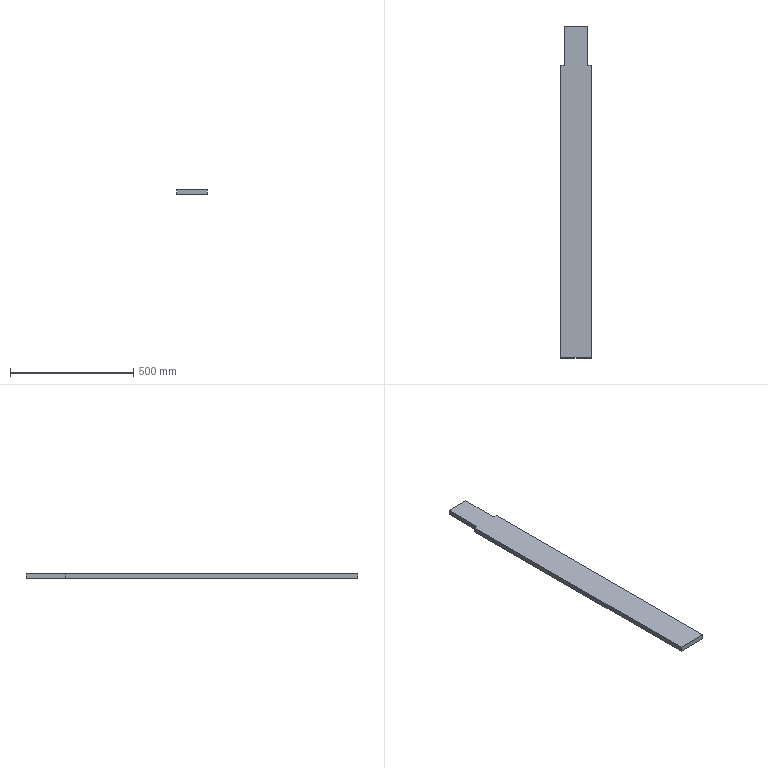Part | STEP file | 01 Counterweight block | 1 solid | 10 faces | box 124 x 1345 x 20 mm | volume 3242800 mm3 | plane 10
STEP:
#1=CARTESIAN_POINT('',(0.,0.,0.));
#2=DIRECTION('',(0.,0.,1.));
#3=DIRECTION('',(1.,0.,0.));
#4=AXIS2_PLACEMENT_3D('',#1,#2,#3);
#5=CARTESIAN_POINT('',(0.,1185.,0.));
#6=VERTEX_POINT('',#5);
#7=CARTESIAN_POINT('',(0.,0.,0.));
#8=VERTEX_POINT('',#7);
#9=CARTESIAN_POINT('',(0.,0.,0.));
#10=DIRECTION('',(0.,-1.,0.));
#11=VECTOR('',#10,1.);
#12=LINE('',#9,#11);
#13=CARTESIAN_POINT('',(0.,0.,20.));
#14=DIRECTION('',(1.,0.,0.));
#15=DIRECTION('',(0.,0.,-1.));
#16=AXIS2_PLACEMENT_3D('',#13,#14,#15);
#17=PLANE('',#16);
#18=CARTESIAN_POINT('',(20.,0.));
#19=DIRECTION('',(0.,-1.));
#20=VECTOR('',#19,1.);
#21=LINE('',#18,#20);
#22=(GEOMETRIC_REPRESENTATION_CONTEXT(2)PARAMETRIC_REPRESENTATION_CONTEXT()REPRESENTATION_CONTEXT('',''));
#23=DEFINITIONAL_REPRESENTATION('',(#21),#22);
#24=PCURVE('',#17,#23);
#25=CARTESIAN_POINT('',(0.,0.,0.));
#26=DIRECTION('',(0.,0.,1.));
#27=DIRECTION('',(1.,0.,0.));
#28=AXIS2_PLACEMENT_3D('',#25,#26,#27);
#29=PLANE('',#28);
#30=CARTESIAN_POINT('',(0.,0.));
#31=DIRECTION('',(0.,-1.));
#32=VECTOR('',#31,1.);
#33=LINE('',#30,#32);
#34=(GEOMETRIC_REPRESENTATION_CONTEXT(2)PARAMETRIC_REPRESENTATION_CONTEXT()REPRESENTATION_CONTEXT('',''));
#35=DEFINITIONAL_REPRESENTATION('',(#33),#34);
#36=PCURVE('',#29,#35);
#37=SURFACE_CURVE('',#12,(#24,#36),.PCURVE_S1.);
#38=EDGE_CURVE('',#6,#8,#37,.T.);
#39=ORIENTED_EDGE('',*,*,#38,.T.);
#40=CARTESIAN_POINT('',(0.,0.,20.));
#41=VERTEX_POINT('',#40);
#42=CARTESIAN_POINT('',(0.,0.,20.));
#43=DIRECTION('',(0.,0.,-1.));
#44=VECTOR('',#43,1.);
#45=LINE('',#42,#44);
#46=CARTESIAN_POINT('',(0.,0.));
#47=DIRECTION('',(1.,0.));
#48=VECTOR('',#47,1.);
#49=LINE('',#46,#48);
#50=(GEOMETRIC_REPRESENTATION_CONTEXT(2)PARAMETRIC_REPRESENTATION_CONTEXT()REPRESENTATION_CONTEXT('',''));
#51=DEFINITIONAL_REPRESENTATION('',(#49),#50);
#52=PCURVE('',#17,#51);
#53=CARTESIAN_POINT('',(0.,0.,20.));
#54=DIRECTION('',(0.,1.,0.));
#55=DIRECTION('',(0.,0.,1.));
#56=AXIS2_PLACEMENT_3D('',#53,#54,#55);
#57=PLANE('',#56);
#58=CARTESIAN_POINT('',(0.,0.));
#59=DIRECTION('',(-1.,0.));
#60=VECTOR('',#59,1.);
#61=LINE('',#58,#60);
#62=(GEOMETRIC_REPRESENTATION_CONTEXT(2)PARAMETRIC_REPRESENTATION_CONTEXT()REPRESENTATION_CONTEXT('',''));
#63=DEFINITIONAL_REPRESENTATION('',(#61),#62);
#64=PCURVE('',#57,#63);
#65=SURFACE_CURVE('',#45,(#52,#64),.PCURVE_S1.);
#66=EDGE_CURVE('',#41,#8,#65,.T.);
#67=ORIENTED_EDGE('',*,*,#66,.F.);
#68=CARTESIAN_POINT('',(0.,1185.,20.));
#69=VERTEX_POINT('',#68);
#70=CARTESIAN_POINT('',(0.,0.,20.));
#71=DIRECTION('',(0.,-1.,0.));
#72=VECTOR('',#71,1.);
#73=LINE('',#70,#72);
#74=CARTESIAN_POINT('',(0.,0.));
#75=DIRECTION('',(0.,-1.));
#76=VECTOR('',#75,1.);
#77=LINE('',#74,#76);
#78=(GEOMETRIC_REPRESENTATION_CONTEXT(2)PARAMETRIC_REPRESENTATION_CONTEXT()REPRESENTATION_CONTEXT('',''));
#79=DEFINITIONAL_REPRESENTATION('',(#77),#78);
#80=PCURVE('',#17,#79);
#81=CARTESIAN_POINT('',(0.,0.,20.));
#82=DIRECTION('',(0.,0.,1.));
#83=DIRECTION('',(1.,0.,0.));
#84=AXIS2_PLACEMENT_3D('',#81,#82,#83);
#85=PLANE('',#84);
#86=CARTESIAN_POINT('',(0.,0.));
#87=DIRECTION('',(0.,-1.));
#88=VECTOR('',#87,1.);
#89=LINE('',#86,#88);
#90=(GEOMETRIC_REPRESENTATION_CONTEXT(2)PARAMETRIC_REPRESENTATION_CONTEXT()REPRESENTATION_CONTEXT('',''));
#91=DEFINITIONAL_REPRESENTATION('',(#89),#90);
#92=PCURVE('',#85,#91);
#93=SURFACE_CURVE('',#73,(#80,#92),.PCURVE_S1.);
#94=EDGE_CURVE('',#69,#41,#93,.T.);
#95=ORIENTED_EDGE('',*,*,#94,.F.);
#96=CARTESIAN_POINT('',(0.,1185.,20.));
#97=DIRECTION('',(0.,0.,-1.));
#98=VECTOR('',#97,1.);
#99=LINE('',#96,#98);
#100=CARTESIAN_POINT('',(0.,1185.));
#101=DIRECTION('',(1.,0.));
#102=VECTOR('',#101,1.);
#103=LINE('',#100,#102);
#104=(GEOMETRIC_REPRESENTATION_CONTEXT(2)PARAMETRIC_REPRESENTATION_CONTEXT()REPRESENTATION_CONTEXT('',''));
#105=DEFINITIONAL_REPRESENTATION('',(#103),#104);
#106=PCURVE('',#17,#105);
#107=CARTESIAN_POINT('',(14.5,1185.,20.));
#108=DIRECTION('',(0.,-1.,0.));
#109=DIRECTION('',(0.,0.,-1.));
#110=AXIS2_PLACEMENT_3D('',#107,#108,#109);
#111=PLANE('',#110);
#112=CARTESIAN_POINT('',(0.,-14.5));
#113=DIRECTION('',(1.,0.));
#114=VECTOR('',#113,1.);
#115=LINE('',#112,#114);
#116=(GEOMETRIC_REPRESENTATION_CONTEXT(2)PARAMETRIC_REPRESENTATION_CONTEXT()REPRESENTATION_CONTEXT('',''));
#117=DEFINITIONAL_REPRESENTATION('',(#115),#116);
#118=PCURVE('',#111,#117);
#119=SURFACE_CURVE('',#99,(#106,#118),.PCURVE_S1.);
#120=EDGE_CURVE('',#69,#6,#119,.T.);
#121=ORIENTED_EDGE('',*,*,#120,.T.);
#122=EDGE_LOOP('',(#39,#67,#95,#121));
#123=FACE_BOUND('',#122,.T.);
#124=ADVANCED_FACE('',(#123),#17,.F.);
#125=CARTESIAN_POINT('',(124.,0.,0.));
#126=VERTEX_POINT('',#125);
#127=CARTESIAN_POINT('',(0.,0.,0.));
#128=DIRECTION('',(1.,0.,0.));
#129=VECTOR('',#128,1.);
#130=LINE('',#127,#129);
#131=CARTESIAN_POINT('',(-20.,0.));
#132=DIRECTION('',(0.,1.));
#133=VECTOR('',#132,1.);
#134=LINE('',#131,#133);
#135=(GEOMETRIC_REPRESENTATION_CONTEXT(2)PARAMETRIC_REPRESENTATION_CONTEXT()REPRESENTATION_CONTEXT('',''));
#136=DEFINITIONAL_REPRESENTATION('',(#134),#135);
#137=PCURVE('',#57,#136);
#138=CARTESIAN_POINT('',(0.,0.));
#139=DIRECTION('',(1.,0.));
#140=VECTOR('',#139,1.);
#141=LINE('',#138,#140);
#142=(GEOMETRIC_REPRESENTATION_CONTEXT(2)PARAMETRIC_REPRESENTATION_CONTEXT()REPRESENTATION_CONTEXT('',''));
#143=DEFINITIONAL_REPRESENTATION('',(#141),#142);
#144=PCURVE('',#29,#143);
#145=SURFACE_CURVE('',#130,(#137,#144),.PCURVE_S1.);
#146=EDGE_CURVE('',#8,#126,#145,.T.);
#147=ORIENTED_EDGE('',*,*,#146,.T.);
#148=CARTESIAN_POINT('',(124.,0.,20.));
#149=VERTEX_POINT('',#148);
#150=CARTESIAN_POINT('',(124.,0.,20.));
#151=DIRECTION('',(0.,0.,-1.));
#152=VECTOR('',#151,1.);
#153=LINE('',#150,#152);
#154=CARTESIAN_POINT('',(0.,124.));
#155=DIRECTION('',(-1.,0.));
#156=VECTOR('',#155,1.);
#157=LINE('',#154,#156);
#158=(GEOMETRIC_REPRESENTATION_CONTEXT(2)PARAMETRIC_REPRESENTATION_CONTEXT()REPRESENTATION_CONTEXT('',''));
#159=DEFINITIONAL_REPRESENTATION('',(#157),#158);
#160=PCURVE('',#57,#159);
#161=CARTESIAN_POINT('',(124.,0.,20.));
#162=DIRECTION('',(-1.,0.,0.));
#163=DIRECTION('',(0.,0.,1.));
#164=AXIS2_PLACEMENT_3D('',#161,#162,#163);
#165=PLANE('',#164);
#166=CARTESIAN_POINT('',(0.,0.));
#167=DIRECTION('',(-1.,0.));
#168=VECTOR('',#167,1.);
#169=LINE('',#166,#168);
#170=(GEOMETRIC_REPRESENTATION_CONTEXT(2)PARAMETRIC_REPRESENTATION_CONTEXT()REPRESENTATION_CONTEXT('',''));
#171=DEFINITIONAL_REPRESENTATION('',(#169),#170);
#172=PCURVE('',#165,#171);
#173=SURFACE_CURVE('',#153,(#160,#172),.PCURVE_S1.);
#174=EDGE_CURVE('',#149,#126,#173,.T.);
#175=ORIENTED_EDGE('',*,*,#174,.F.);
#176=CARTESIAN_POINT('',(0.,0.,20.));
#177=DIRECTION('',(1.,0.,0.));
#178=VECTOR('',#177,1.);
#179=LINE('',#176,#178);
#180=CARTESIAN_POINT('',(0.,0.));
#181=DIRECTION('',(0.,1.));
#182=VECTOR('',#181,1.);
#183=LINE('',#180,#182);
#184=(GEOMETRIC_REPRESENTATION_CONTEXT(2)PARAMETRIC_REPRESENTATION_CONTEXT()REPRESENTATION_CONTEXT('',''));
#185=DEFINITIONAL_REPRESENTATION('',(#183),#184);
#186=PCURVE('',#57,#185);
#187=CARTESIAN_POINT('',(0.,0.));
#188=DIRECTION('',(1.,0.));
#189=VECTOR('',#188,1.);
#190=LINE('',#187,#189);
#191=(GEOMETRIC_REPRESENTATION_CONTEXT(2)PARAMETRIC_REPRESENTATION_CONTEXT()REPRESENTATION_CONTEXT('',''));
#192=DEFINITIONAL_REPRESENTATION('',(#190),#191);
#193=PCURVE('',#85,#192);
#194=SURFACE_CURVE('',#179,(#186,#193),.PCURVE_S1.);
#195=EDGE_CURVE('',#41,#149,#194,.T.);
#196=ORIENTED_EDGE('',*,*,#195,.F.);
#197=ORIENTED_EDGE('',*,*,#66,.T.);
#198=EDGE_LOOP('',(#147,#175,#196,#197));
#199=FACE_BOUND('',#198,.T.);
#200=ADVANCED_FACE('',(#199),#57,.F.);
#201=CARTESIAN_POINT('',(124.,1185.,0.));
#202=VERTEX_POINT('',#201);
#203=CARTESIAN_POINT('',(124.,0.,0.));
#204=DIRECTION('',(0.,1.,0.));
#205=VECTOR('',#204,1.);
#206=LINE('',#203,#205);
#207=CARTESIAN_POINT('',(-20.,0.));
#208=DIRECTION('',(0.,1.));
#209=VECTOR('',#208,1.);
#210=LINE('',#207,#209);
#211=(GEOMETRIC_REPRESENTATION_CONTEXT(2)PARAMETRIC_REPRESENTATION_CONTEXT()REPRESENTATION_CONTEXT('',''));
#212=DEFINITIONAL_REPRESENTATION('',(#210),#211);
#213=PCURVE('',#165,#212);
#214=CARTESIAN_POINT('',(124.,0.));
#215=DIRECTION('',(0.,1.));
#216=VECTOR('',#215,1.);
#217=LINE('',#214,#216);
#218=(GEOMETRIC_REPRESENTATION_CONTEXT(2)PARAMETRIC_REPRESENTATION_CONTEXT()REPRESENTATION_CONTEXT('',''));
#219=DEFINITIONAL_REPRESENTATION('',(#217),#218);
#220=PCURVE('',#29,#219);
#221=SURFACE_CURVE('',#206,(#213,#220),.PCURVE_S1.);
#222=EDGE_CURVE('',#126,#202,#221,.T.);
#223=ORIENTED_EDGE('',*,*,#222,.T.);
#224=CARTESIAN_POINT('',(124.,1185.,20.));
#225=VERTEX_POINT('',#224);
#226=CARTESIAN_POINT('',(124.,1185.,20.));
#227=DIRECTION('',(0.,0.,-1.));
#228=VECTOR('',#227,1.);
#229=LINE('',#226,#228);
#230=CARTESIAN_POINT('',(0.,1185.));
#231=DIRECTION('',(-1.,0.));
#232=VECTOR('',#231,1.);
#233=LINE('',#230,#232);
#234=(GEOMETRIC_REPRESENTATION_CONTEXT(2)PARAMETRIC_REPRESENTATION_CONTEXT()REPRESENTATION_CONTEXT('',''));
#235=DEFINITIONAL_REPRESENTATION('',(#233),#234);
#236=PCURVE('',#165,#235);
#237=CARTESIAN_POINT('',(109.5,1185.,20.));
#238=DIRECTION('',(0.,-1.,0.));
#239=DIRECTION('',(0.,0.,-1.));
#240=AXIS2_PLACEMENT_3D('',#237,#238,#239);
#241=PLANE('',#240);
#242=CARTESIAN_POINT('',(0.,14.5));
#243=DIRECTION('',(1.,0.));
#244=VECTOR('',#243,1.);
#245=LINE('',#242,#244);
#246=(GEOMETRIC_REPRESENTATION_CONTEXT(2)PARAMETRIC_REPRESENTATION_CONTEXT()REPRESENTATION_CONTEXT('',''));
#247=DEFINITIONAL_REPRESENTATION('',(#245),#246);
#248=PCURVE('',#241,#247);
#249=SURFACE_CURVE('',#229,(#236,#248),.PCURVE_S1.);
#250=EDGE_CURVE('',#225,#202,#249,.T.);
#251=ORIENTED_EDGE('',*,*,#250,.F.);
#252=CARTESIAN_POINT('',(124.,0.,20.));
#253=DIRECTION('',(0.,1.,0.));
#254=VECTOR('',#253,1.);
#255=LINE('',#252,#254);
#256=CARTESIAN_POINT('',(0.,0.));
#257=DIRECTION('',(0.,1.));
#258=VECTOR('',#257,1.);
#259=LINE('',#256,#258);
#260=(GEOMETRIC_REPRESENTATION_CONTEXT(2)PARAMETRIC_REPRESENTATION_CONTEXT()REPRESENTATION_CONTEXT('',''));
#261=DEFINITIONAL_REPRESENTATION('',(#259),#260);
#262=PCURVE('',#165,#261);
#263=CARTESIAN_POINT('',(124.,0.));
#264=DIRECTION('',(0.,1.));
#265=VECTOR('',#264,1.);
#266=LINE('',#263,#265);
#267=(GEOMETRIC_REPRESENTATION_CONTEXT(2)PARAMETRIC_REPRESENTATION_CONTEXT()REPRESENTATION_CONTEXT('',''));
#268=DEFINITIONAL_REPRESENTATION('',(#266),#267);
#269=PCURVE('',#85,#268);
#270=SURFACE_CURVE('',#255,(#262,#269),.PCURVE_S1.);
#271=EDGE_CURVE('',#149,#225,#270,.T.);
#272=ORIENTED_EDGE('',*,*,#271,.F.);
#273=ORIENTED_EDGE('',*,*,#174,.T.);
#274=EDGE_LOOP('',(#223,#251,#272,#273));
#275=FACE_BOUND('',#274,.T.);
#276=ADVANCED_FACE('',(#275),#165,.F.);
#277=CARTESIAN_POINT('',(109.5,1185.,0.));
#278=VERTEX_POINT('',#277);
#279=CARTESIAN_POINT('',(109.5,1185.,0.));
#280=DIRECTION('',(-1.,0.,0.));
#281=VECTOR('',#280,1.);
#282=LINE('',#279,#281);
#283=CARTESIAN_POINT('',(20.,0.));
#284=DIRECTION('',(0.,-1.));
#285=VECTOR('',#284,1.);
#286=LINE('',#283,#285);
#287=(GEOMETRIC_REPRESENTATION_CONTEXT(2)PARAMETRIC_REPRESENTATION_CONTEXT()REPRESENTATION_CONTEXT('',''));
#288=DEFINITIONAL_REPRESENTATION('',(#286),#287);
#289=PCURVE('',#241,#288);
#290=CARTESIAN_POINT('',(109.5,1185.));
#291=DIRECTION('',(-1.,0.));
#292=VECTOR('',#291,1.);
#293=LINE('',#290,#292);
#294=(GEOMETRIC_REPRESENTATION_CONTEXT(2)PARAMETRIC_REPRESENTATION_CONTEXT()REPRESENTATION_CONTEXT('',''));
#295=DEFINITIONAL_REPRESENTATION('',(#293),#294);
#296=PCURVE('',#29,#295);
#297=SURFACE_CURVE('',#282,(#289,#296),.PCURVE_S1.);
#298=EDGE_CURVE('',#202,#278,#297,.T.);
#299=ORIENTED_EDGE('',*,*,#298,.T.);
#300=CARTESIAN_POINT('',(109.5,1185.,20.));
#301=VERTEX_POINT('',#300);
#302=CARTESIAN_POINT('',(109.5,1185.,20.));
#303=DIRECTION('',(0.,0.,-1.));
#304=VECTOR('',#303,1.);
#305=LINE('',#302,#304);
#306=CARTESIAN_POINT('',(0.,0.));
#307=DIRECTION('',(1.,0.));
#308=VECTOR('',#307,1.);
#309=LINE('',#306,#308);
#310=(GEOMETRIC_REPRESENTATION_CONTEXT(2)PARAMETRIC_REPRESENTATION_CONTEXT()REPRESENTATION_CONTEXT('',''));
#311=DEFINITIONAL_REPRESENTATION('',(#309),#310);
#312=PCURVE('',#241,#311);
#313=CARTESIAN_POINT('',(109.5,1345.,20.));
#314=DIRECTION('',(-1.,0.,0.));
#315=DIRECTION('',(0.,0.,1.));
#316=AXIS2_PLACEMENT_3D('',#313,#314,#315);
#317=PLANE('',#316);
#318=CARTESIAN_POINT('',(0.,-160.));
#319=DIRECTION('',(-1.,0.));
#320=VECTOR('',#319,1.);
#321=LINE('',#318,#320);
#322=(GEOMETRIC_REPRESENTATION_CONTEXT(2)PARAMETRIC_REPRESENTATION_CONTEXT()REPRESENTATION_CONTEXT('',''));
#323=DEFINITIONAL_REPRESENTATION('',(#321),#322);
#324=PCURVE('',#317,#323);
#325=SURFACE_CURVE('',#305,(#312,#324),.PCURVE_S1.);
#326=EDGE_CURVE('',#301,#278,#325,.T.);
#327=ORIENTED_EDGE('',*,*,#326,.F.);
#328=CARTESIAN_POINT('',(109.5,1185.,20.));
#329=DIRECTION('',(-1.,0.,0.));
#330=VECTOR('',#329,1.);
#331=LINE('',#328,#330);
#332=CARTESIAN_POINT('',(0.,0.));
#333=DIRECTION('',(0.,-1.));
#334=VECTOR('',#333,1.);
#335=LINE('',#332,#334);
#336=(GEOMETRIC_REPRESENTATION_CONTEXT(2)PARAMETRIC_REPRESENTATION_CONTEXT()REPRESENTATION_CONTEXT('',''));
#337=DEFINITIONAL_REPRESENTATION('',(#335),#336);
#338=PCURVE('',#241,#337);
#339=CARTESIAN_POINT('',(109.5,1185.));
#340=DIRECTION('',(-1.,0.));
#341=VECTOR('',#340,1.);
#342=LINE('',#339,#341);
#343=(GEOMETRIC_REPRESENTATION_CONTEXT(2)PARAMETRIC_REPRESENTATION_CONTEXT()REPRESENTATION_CONTEXT('',''));
#344=DEFINITIONAL_REPRESENTATION('',(#342),#343);
#345=PCURVE('',#85,#344);
#346=SURFACE_CURVE('',#331,(#338,#345),.PCURVE_S1.);
#347=EDGE_CURVE('',#225,#301,#346,.T.);
#348=ORIENTED_EDGE('',*,*,#347,.F.);
#349=ORIENTED_EDGE('',*,*,#250,.T.);
#350=EDGE_LOOP('',(#299,#327,#348,#349));
#351=FACE_BOUND('',#350,.T.);
#352=ADVANCED_FACE('',(#351),#241,.F.);
#353=CARTESIAN_POINT('',(109.5,1345.,0.));
#354=VERTEX_POINT('',#353);
#355=CARTESIAN_POINT('',(109.5,1345.,0.));
#356=DIRECTION('',(0.,1.,0.));
#357=VECTOR('',#356,1.);
#358=LINE('',#355,#357);
#359=CARTESIAN_POINT('',(-20.,0.));
#360=DIRECTION('',(0.,1.));
#361=VECTOR('',#360,1.);
#362=LINE('',#359,#361);
#363=(GEOMETRIC_REPRESENTATION_CONTEXT(2)PARAMETRIC_REPRESENTATION_CONTEXT()REPRESENTATION_CONTEXT('',''));
#364=DEFINITIONAL_REPRESENTATION('',(#362),#363);
#365=PCURVE('',#317,#364);
#366=CARTESIAN_POINT('',(109.5,1345.));
#367=DIRECTION('',(0.,1.));
#368=VECTOR('',#367,1.);
#369=LINE('',#366,#368);
#370=(GEOMETRIC_REPRESENTATION_CONTEXT(2)PARAMETRIC_REPRESENTATION_CONTEXT()REPRESENTATION_CONTEXT('',''));
#371=DEFINITIONAL_REPRESENTATION('',(#369),#370);
#372=PCURVE('',#29,#371);
#373=SURFACE_CURVE('',#358,(#365,#372),.PCURVE_S1.);
#374=EDGE_CURVE('',#278,#354,#373,.T.);
#375=ORIENTED_EDGE('',*,*,#374,.T.);
#376=CARTESIAN_POINT('',(109.5,1345.,20.));
#377=VERTEX_POINT('',#376);
#378=CARTESIAN_POINT('',(109.5,1345.,20.));
#379=DIRECTION('',(0.,0.,-1.));
#380=VECTOR('',#379,1.);
#381=LINE('',#378,#380);
#382=CARTESIAN_POINT('',(0.,0.));
#383=DIRECTION('',(-1.,0.));
#384=VECTOR('',#383,1.);
#385=LINE('',#382,#384);
#386=(GEOMETRIC_REPRESENTATION_CONTEXT(2)PARAMETRIC_REPRESENTATION_CONTEXT()REPRESENTATION_CONTEXT('',''));
#387=DEFINITIONAL_REPRESENTATION('',(#385),#386);
#388=PCURVE('',#317,#387);
#389=CARTESIAN_POINT('',(14.5,1345.,20.));
#390=DIRECTION('',(0.,-1.,0.));
#391=DIRECTION('',(0.,0.,-1.));
#392=AXIS2_PLACEMENT_3D('',#389,#390,#391);
#393=PLANE('',#392);
#394=CARTESIAN_POINT('',(0.,95.));
#395=DIRECTION('',(1.,0.));
#396=VECTOR('',#395,1.);
#397=LINE('',#394,#396);
#398=(GEOMETRIC_REPRESENTATION_CONTEXT(2)PARAMETRIC_REPRESENTATION_CONTEXT()REPRESENTATION_CONTEXT('',''));
#399=DEFINITIONAL_REPRESENTATION('',(#397),#398);
#400=PCURVE('',#393,#399);
#401=SURFACE_CURVE('',#381,(#388,#400),.PCURVE_S1.);
#402=EDGE_CURVE('',#377,#354,#401,.T.);
#403=ORIENTED_EDGE('',*,*,#402,.F.);
#404=CARTESIAN_POINT('',(109.5,1345.,20.));
#405=DIRECTION('',(0.,1.,0.));
#406=VECTOR('',#405,1.);
#407=LINE('',#404,#406);
#408=CARTESIAN_POINT('',(0.,0.));
#409=DIRECTION('',(0.,1.));
#410=VECTOR('',#409,1.);
#411=LINE('',#408,#410);
#412=(GEOMETRIC_REPRESENTATION_CONTEXT(2)PARAMETRIC_REPRESENTATION_CONTEXT()REPRESENTATION_CONTEXT('',''));
#413=DEFINITIONAL_REPRESENTATION('',(#411),#412);
#414=PCURVE('',#317,#413);
#415=CARTESIAN_POINT('',(109.5,1345.));
#416=DIRECTION('',(0.,1.));
#417=VECTOR('',#416,1.);
#418=LINE('',#415,#417);
#419=(GEOMETRIC_REPRESENTATION_CONTEXT(2)PARAMETRIC_REPRESENTATION_CONTEXT()REPRESENTATION_CONTEXT('',''));
#420=DEFINITIONAL_REPRESENTATION('',(#418),#419);
#421=PCURVE('',#85,#420);
#422=SURFACE_CURVE('',#407,(#414,#421),.PCURVE_S1.);
#423=EDGE_CURVE('',#301,#377,#422,.T.);
#424=ORIENTED_EDGE('',*,*,#423,.F.);
#425=ORIENTED_EDGE('',*,*,#326,.T.);
#426=EDGE_LOOP('',(#375,#403,#424,#425));
#427=FACE_BOUND('',#426,.T.);
#428=ADVANCED_FACE('',(#427),#317,.F.);
#429=CARTESIAN_POINT('',(14.5,1345.,0.));
#430=VERTEX_POINT('',#429);
#431=CARTESIAN_POINT('',(14.5,1345.,0.));
#432=DIRECTION('',(-1.,0.,0.));
#433=VECTOR('',#432,1.);
#434=LINE('',#431,#433);
#435=CARTESIAN_POINT('',(20.,0.));
#436=DIRECTION('',(0.,-1.));
#437=VECTOR('',#436,1.);
#438=LINE('',#435,#437);
#439=(GEOMETRIC_REPRESENTATION_CONTEXT(2)PARAMETRIC_REPRESENTATION_CONTEXT()REPRESENTATION_CONTEXT('',''));
#440=DEFINITIONAL_REPRESENTATION('',(#438),#439);
#441=PCURVE('',#393,#440);
#442=CARTESIAN_POINT('',(14.5,1345.));
#443=DIRECTION('',(-1.,0.));
#444=VECTOR('',#443,1.);
#445=LINE('',#442,#444);
#446=(GEOMETRIC_REPRESENTATION_CONTEXT(2)PARAMETRIC_REPRESENTATION_CONTEXT()REPRESENTATION_CONTEXT('',''));
#447=DEFINITIONAL_REPRESENTATION('',(#445),#446);
#448=PCURVE('',#29,#447);
#449=SURFACE_CURVE('',#434,(#441,#448),.PCURVE_S1.);
#450=EDGE_CURVE('',#354,#430,#449,.T.);
#451=ORIENTED_EDGE('',*,*,#450,.T.);
#452=CARTESIAN_POINT('',(14.5,1345.,20.));
#453=VERTEX_POINT('',#452);
#454=CARTESIAN_POINT('',(14.5,1345.,20.));
#455=DIRECTION('',(0.,0.,-1.));
#456=VECTOR('',#455,1.);
#457=LINE('',#454,#456);
#458=CARTESIAN_POINT('',(0.,0.));
#459=DIRECTION('',(1.,0.));
#460=VECTOR('',#459,1.);
#461=LINE('',#458,#460);
#462=(GEOMETRIC_REPRESENTATION_CONTEXT(2)PARAMETRIC_REPRESENTATION_CONTEXT()REPRESENTATION_CONTEXT('',''));
#463=DEFINITIONAL_REPRESENTATION('',(#461),#462);
#464=PCURVE('',#393,#463);
#465=CARTESIAN_POINT('',(14.5,1345.,20.));
#466=DIRECTION('',(1.,0.,0.));
#467=DIRECTION('',(0.,1.,0.));
#468=AXIS2_PLACEMENT_3D('',#465,#466,#467);
#469=PLANE('',#468);
#470=CARTESIAN_POINT('',(0.,0.));
#471=DIRECTION('',(0.,-1.));
#472=VECTOR('',#471,1.);
#473=LINE('',#470,#472);
#474=(GEOMETRIC_REPRESENTATION_CONTEXT(2)PARAMETRIC_REPRESENTATION_CONTEXT()REPRESENTATION_CONTEXT('',''));
#475=DEFINITIONAL_REPRESENTATION('',(#473),#474);
#476=PCURVE('',#469,#475);
#477=SURFACE_CURVE('',#457,(#464,#476),.PCURVE_S1.);
#478=EDGE_CURVE('',#453,#430,#477,.T.);
#479=ORIENTED_EDGE('',*,*,#478,.F.);
#480=CARTESIAN_POINT('',(14.5,1345.,20.));
#481=DIRECTION('',(-1.,0.,0.));
#482=VECTOR('',#481,1.);
#483=LINE('',#480,#482);
#484=CARTESIAN_POINT('',(0.,0.));
#485=DIRECTION('',(0.,-1.));
#486=VECTOR('',#485,1.);
#487=LINE('',#484,#486);
#488=(GEOMETRIC_REPRESENTATION_CONTEXT(2)PARAMETRIC_REPRESENTATION_CONTEXT()REPRESENTATION_CONTEXT('',''));
#489=DEFINITIONAL_REPRESENTATION('',(#487),#488);
#490=PCURVE('',#393,#489);
#491=CARTESIAN_POINT('',(14.5,1345.));
#492=DIRECTION('',(-1.,0.));
#493=VECTOR('',#492,1.);
#494=LINE('',#491,#493);
#495=(GEOMETRIC_REPRESENTATION_CONTEXT(2)PARAMETRIC_REPRESENTATION_CONTEXT()REPRESENTATION_CONTEXT('',''));
#496=DEFINITIONAL_REPRESENTATION('',(#494),#495);
#497=PCURVE('',#85,#496);
#498=SURFACE_CURVE('',#483,(#490,#497),.PCURVE_S1.);
#499=EDGE_CURVE('',#377,#453,#498,.T.);
#500=ORIENTED_EDGE('',*,*,#499,.F.);
#501=ORIENTED_EDGE('',*,*,#402,.T.);
#502=EDGE_LOOP('',(#451,#479,#500,#501));
#503=FACE_BOUND('',#502,.T.);
#504=ADVANCED_FACE('',(#503),#393,.F.);
#505=CARTESIAN_POINT('',(14.5,1185.,0.));
#506=VERTEX_POINT('',#505);
#507=CARTESIAN_POINT('',(14.5,1345.,0.));
#508=DIRECTION('',(0.,-1.,0.));
#509=VECTOR('',#508,1.);
#510=LINE('',#507,#509);
#511=CARTESIAN_POINT('',(0.,-20.));
#512=DIRECTION('',(-1.,0.));
#513=VECTOR('',#512,1.);
#514=LINE('',#511,#513);
#515=(GEOMETRIC_REPRESENTATION_CONTEXT(2)PARAMETRIC_REPRESENTATION_CONTEXT()REPRESENTATION_CONTEXT('',''));
#516=DEFINITIONAL_REPRESENTATION('',(#514),#515);
#517=PCURVE('',#469,#516);
#518=CARTESIAN_POINT('',(14.5,1345.));
#519=DIRECTION('',(0.,-1.));
#520=VECTOR('',#519,1.);
#521=LINE('',#518,#520);
#522=(GEOMETRIC_REPRESENTATION_CONTEXT(2)PARAMETRIC_REPRESENTATION_CONTEXT()REPRESENTATION_CONTEXT('',''));
#523=DEFINITIONAL_REPRESENTATION('',(#521),#522);
#524=PCURVE('',#29,#523);
#525=SURFACE_CURVE('',#510,(#517,#524),.PCURVE_S1.);
#526=EDGE_CURVE('',#430,#506,#525,.T.);
#527=ORIENTED_EDGE('',*,*,#526,.T.);
#528=CARTESIAN_POINT('',(14.5,1185.,20.));
#529=VERTEX_POINT('',#528);
#530=CARTESIAN_POINT('',(14.5,1185.,20.));
#531=DIRECTION('',(0.,0.,-1.));
#532=VECTOR('',#531,1.);
#533=LINE('',#530,#532);
#534=CARTESIAN_POINT('',(-160.,0.));
#535=DIRECTION('',(0.,-1.));
#536=VECTOR('',#535,1.);
#537=LINE('',#534,#536);
#538=(GEOMETRIC_REPRESENTATION_CONTEXT(2)PARAMETRIC_REPRESENTATION_CONTEXT()REPRESENTATION_CONTEXT('',''));
#539=DEFINITIONAL_REPRESENTATION('',(#537),#538);
#540=PCURVE('',#469,#539);
#541=CARTESIAN_POINT('',(0.,0.));
#542=DIRECTION('',(1.,0.));
#543=VECTOR('',#542,1.);
#544=LINE('',#541,#543);
#545=(GEOMETRIC_REPRESENTATION_CONTEXT(2)PARAMETRIC_REPRESENTATION_CONTEXT()REPRESENTATION_CONTEXT('',''));
#546=DEFINITIONAL_REPRESENTATION('',(#544),#545);
#547=PCURVE('',#111,#546);
#548=SURFACE_CURVE('',#533,(#540,#547),.PCURVE_S1.);
#549=EDGE_CURVE('',#529,#506,#548,.T.);
#550=ORIENTED_EDGE('',*,*,#549,.F.);
#551=CARTESIAN_POINT('',(14.5,1345.,20.));
#552=DIRECTION('',(0.,-1.,0.));
#553=VECTOR('',#552,1.);
#554=LINE('',#551,#553);
#555=CARTESIAN_POINT('',(0.,0.));
#556=DIRECTION('',(-1.,0.));
#557=VECTOR('',#556,1.);
#558=LINE('',#555,#557);
#559=(GEOMETRIC_REPRESENTATION_CONTEXT(2)PARAMETRIC_REPRESENTATION_CONTEXT()REPRESENTATION_CONTEXT('',''));
#560=DEFINITIONAL_REPRESENTATION('',(#558),#559);
#561=PCURVE('',#469,#560);
#562=CARTESIAN_POINT('',(14.5,1345.));
#563=DIRECTION('',(0.,-1.));
#564=VECTOR('',#563,1.);
#565=LINE('',#562,#564);
#566=(GEOMETRIC_REPRESENTATION_CONTEXT(2)PARAMETRIC_REPRESENTATION_CONTEXT()REPRESENTATION_CONTEXT('',''));
#567=DEFINITIONAL_REPRESENTATION('',(#565),#566);
#568=PCURVE('',#85,#567);
#569=SURFACE_CURVE('',#554,(#561,#568),.PCURVE_S1.);
#570=EDGE_CURVE('',#453,#529,#569,.T.);
#571=ORIENTED_EDGE('',*,*,#570,.F.);
#572=ORIENTED_EDGE('',*,*,#478,.T.);
#573=EDGE_LOOP('',(#527,#550,#571,#572));
#574=FACE_BOUND('',#573,.T.);
#575=ADVANCED_FACE('',(#574),#469,.F.);
#576=CARTESIAN_POINT('',(14.5,1185.,0.));
#577=DIRECTION('',(-1.,0.,0.));
#578=VECTOR('',#577,1.);
#579=LINE('',#576,#578);
#580=CARTESIAN_POINT('',(20.,0.));
#581=DIRECTION('',(0.,-1.));
#582=VECTOR('',#581,1.);
#583=LINE('',#580,#582);
#584=(GEOMETRIC_REPRESENTATION_CONTEXT(2)PARAMETRIC_REPRESENTATION_CONTEXT()REPRESENTATION_CONTEXT('',''));
#585=DEFINITIONAL_REPRESENTATION('',(#583),#584);
#586=PCURVE('',#111,#585);
#587=CARTESIAN_POINT('',(14.5,1185.));
#588=DIRECTION('',(-1.,0.));
#589=VECTOR('',#588,1.);
#590=LINE('',#587,#589);
#591=(GEOMETRIC_REPRESENTATION_CONTEXT(2)PARAMETRIC_REPRESENTATION_CONTEXT()REPRESENTATION_CONTEXT('',''));
#592=DEFINITIONAL_REPRESENTATION('',(#590),#591);
#593=PCURVE('',#29,#592);
#594=SURFACE_CURVE('',#579,(#586,#593),.PCURVE_S1.);
#595=EDGE_CURVE('',#506,#6,#594,.T.);
#596=ORIENTED_EDGE('',*,*,#595,.T.);
#597=ORIENTED_EDGE('',*,*,#120,.F.);
#598=CARTESIAN_POINT('',(14.5,1185.,20.));
#599=DIRECTION('',(-1.,0.,0.));
#600=VECTOR('',#599,1.);
#601=LINE('',#598,#600);
#602=CARTESIAN_POINT('',(0.,0.));
#603=DIRECTION('',(0.,-1.));
#604=VECTOR('',#603,1.);
#605=LINE('',#602,#604);
#606=(GEOMETRIC_REPRESENTATION_CONTEXT(2)PARAMETRIC_REPRESENTATION_CONTEXT()REPRESENTATION_CONTEXT('',''));
#607=DEFINITIONAL_REPRESENTATION('',(#605),#606);
#608=PCURVE('',#111,#607);
#609=CARTESIAN_POINT('',(14.5,1185.));
#610=DIRECTION('',(-1.,0.));
#611=VECTOR('',#610,1.);
#612=LINE('',#609,#611);
#613=(GEOMETRIC_REPRESENTATION_CONTEXT(2)PARAMETRIC_REPRESENTATION_CONTEXT()REPRESENTATION_CONTEXT('',''));
#614=DEFINITIONAL_REPRESENTATION('',(#612),#613);
#615=PCURVE('',#85,#614);
#616=SURFACE_CURVE('',#601,(#608,#615),.PCURVE_S1.);
#617=EDGE_CURVE('',#529,#69,#616,.T.);
#618=ORIENTED_EDGE('',*,*,#617,.F.);
#619=ORIENTED_EDGE('',*,*,#549,.T.);
#620=EDGE_LOOP('',(#596,#597,#618,#619));
#621=FACE_BOUND('',#620,.T.);
#622=ADVANCED_FACE('',(#621),#111,.F.);
#623=ORIENTED_EDGE('',*,*,#94,.T.);
#624=ORIENTED_EDGE('',*,*,#195,.T.);
#625=ORIENTED_EDGE('',*,*,#271,.T.);
#626=ORIENTED_EDGE('',*,*,#347,.T.);
#627=ORIENTED_EDGE('',*,*,#423,.T.);
#628=ORIENTED_EDGE('',*,*,#499,.T.);
#629=ORIENTED_EDGE('',*,*,#570,.T.);
#630=ORIENTED_EDGE('',*,*,#617,.T.);
#631=EDGE_LOOP('',(#623,#624,#625,#626,#627,#628,#629,#630));
#632=FACE_BOUND('',#631,.T.);
#633=ADVANCED_FACE('',(#632),#85,.T.);
#634=ORIENTED_EDGE('',*,*,#38,.F.);
#635=ORIENTED_EDGE('',*,*,#595,.F.);
#636=ORIENTED_EDGE('',*,*,#526,.F.);
#637=ORIENTED_EDGE('',*,*,#450,.F.);
#638=ORIENTED_EDGE('',*,*,#374,.F.);
#639=ORIENTED_EDGE('',*,*,#298,.F.);
#640=ORIENTED_EDGE('',*,*,#222,.F.);
#641=ORIENTED_EDGE('',*,*,#146,.F.);
#642=EDGE_LOOP('',(#634,#635,#636,#637,#638,#639,#640,#641));
#643=FACE_BOUND('',#642,.T.);
#644=ADVANCED_FACE('',(#643),#29,.F.);
#645=CLOSED_SHELL('',(#124,#200,#276,#352,#428,#504,#575,#622,#633,#644));
#646=MANIFOLD_SOLID_BREP('',#645);
#647=(LENGTH_UNIT()NAMED_UNIT(*)SI_UNIT(.MILLI.,.METRE.));
#648=UNCERTAINTY_MEASURE_WITH_UNIT(LENGTH_MEASURE(0.0000001),#647,'','');
#649=(NAMED_UNIT(*)PLANE_ANGLE_UNIT()SI_UNIT($,.RADIAN.));
#650=(NAMED_UNIT(*)SI_UNIT($,.STERADIAN.)SOLID_ANGLE_UNIT());
#651=(GEOMETRIC_REPRESENTATION_CONTEXT(3)GLOBAL_UNCERTAINTY_ASSIGNED_CONTEXT((#648))GLOBAL_UNIT_ASSIGNED_CONTEXT((#647,#649,#650))REPRESENTATION_CONTEXT('',''));
#652=ADVANCED_BREP_SHAPE_REPRESENTATION('',(#4,#646),#651);